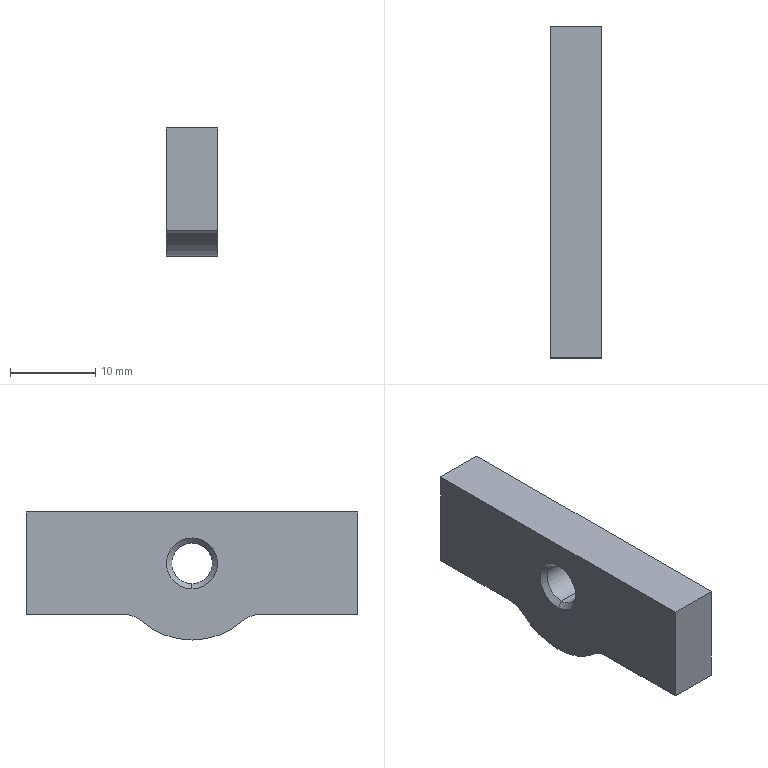Part | STEP file | 2026.6.15-Main Assembly图.sldasm-Part-231 | 1 solid | 17 faces | box 6 x 39 x 15.045 mm | volume 2873 mm3 | plane 7 | cylinder 6 | cone 4 | commonest cylinder face diameters 4.8 x2 6 x2 18 x2
STEP:
#1=CARTESIAN_POINT('',(-1568.238,1430.217,3336.397));
#2=VERTEX_POINT('',#1);
#3=CARTESIAN_POINT('',(-1568.238,1424.264,3334.147));
#4=VERTEX_POINT('',#3);
#5=CARTESIAN_POINT('',(-1568.238,1424.264,3343.147));
#6=DIRECTION('',(-1.,0.,0.));
#7=DIRECTION('',(0.,0.,1.));
#8=AXIS2_PLACEMENT_3D('',#5,#6,#7);
#9=CIRCLE('',#8,9.);
#10=EDGE_CURVE('',#2,#4,#9,.T.);
#11=ORIENTED_EDGE('',*,*,#10,.T.);
#12=CARTESIAN_POINT('',(-1574.238,1424.264,3334.147));
#13=VERTEX_POINT('',#12);
#14=CARTESIAN_POINT('',(-1568.238,1424.264,3334.147));
#15=DIRECTION('',(-1.,0.,0.));
#16=VECTOR('',#15,1000.);
#17=LINE('',#14,#16);
#18=EDGE_CURVE('',#4,#13,#17,.T.);
#19=ORIENTED_EDGE('',*,*,#18,.T.);
#20=CARTESIAN_POINT('',(-1574.238,1430.217,3336.397));
#21=VERTEX_POINT('',#20);
#22=CARTESIAN_POINT('',(-1574.238,1424.264,3343.147));
#23=DIRECTION('',(1.,0.,0.));
#24=DIRECTION('',(0.,0.,1.));
#25=AXIS2_PLACEMENT_3D('',#22,#23,#24);
#26=CIRCLE('',#25,9.);
#27=EDGE_CURVE('',#13,#21,#26,.T.);
#28=ORIENTED_EDGE('',*,*,#27,.T.);
#29=CARTESIAN_POINT('',(-1568.238,1430.217,3336.397));
#30=DIRECTION('',(1.,0.,0.));
#31=VECTOR('',#30,1000.);
#32=LINE('',#29,#31);
#33=EDGE_CURVE('',#21,#2,#32,.T.);
#34=ORIENTED_EDGE('',*,*,#33,.T.);
#35=EDGE_LOOP('',(#11,#19,#28,#34));
#36=FACE_OUTER_BOUND('',#35,.T.);
#37=CARTESIAN_POINT('',(-1568.238,1424.264,3343.147));
#38=DIRECTION('',(-1.,0.,0.));
#39=DIRECTION('',(0.,0.,-1.));
#40=AXIS2_PLACEMENT_3D('',#37,#38,#39);
#41=CYLINDRICAL_SURFACE('',#40,9.);
#42=ADVANCED_FACE('',(#36),#41,.T.);
#43=CARTESIAN_POINT('',(-1568.838,1426.664,3343.147));
#44=VERTEX_POINT('',#43);
#45=CARTESIAN_POINT('',(-1568.238,1427.264,3343.147));
#46=VERTEX_POINT('',#45);
#47=CARTESIAN_POINT('',(-1568.238,1427.264,3343.147));
#48=DIRECTION('',(0.7071,0.7071,0.));
#49=VECTOR('',#48,1000.);
#50=LINE('',#47,#49);
#51=EDGE_CURVE('',#44,#46,#50,.T.);
#52=ORIENTED_EDGE('',*,*,#51,.F.);
#53=CARTESIAN_POINT('',(-1568.838,1424.264,3340.747));
#54=VERTEX_POINT('',#53);
#55=CARTESIAN_POINT('',(-1568.838,1424.264,3343.147));
#56=DIRECTION('',(-1.,0.,0.));
#57=DIRECTION('',(0.,0.,-1.));
#58=AXIS2_PLACEMENT_3D('',#55,#56,#57);
#59=CIRCLE('',#58,2.4);
#60=EDGE_CURVE('',#44,#54,#59,.T.);
#61=ORIENTED_EDGE('',*,*,#60,.T.);
#62=CARTESIAN_POINT('',(-1568.838,1421.864,3343.147));
#63=VERTEX_POINT('',#62);
#64=CARTESIAN_POINT('',(-1568.838,1424.264,3343.147));
#65=DIRECTION('',(-1.,0.,0.));
#66=DIRECTION('',(0.,0.,-1.));
#67=AXIS2_PLACEMENT_3D('',#64,#65,#66);
#68=CIRCLE('',#67,2.4);
#69=EDGE_CURVE('',#54,#63,#68,.T.);
#70=ORIENTED_EDGE('',*,*,#69,.T.);
#71=CARTESIAN_POINT('',(-1568.238,1421.264,3343.147));
#72=VERTEX_POINT('',#71);
#73=CARTESIAN_POINT('',(-1568.238,1421.264,3343.147));
#74=DIRECTION('',(0.7071,-0.7071,0.));
#75=VECTOR('',#74,1000.);
#76=LINE('',#73,#75);
#77=EDGE_CURVE('',#63,#72,#76,.T.);
#78=ORIENTED_EDGE('',*,*,#77,.T.);
#79=CARTESIAN_POINT('',(-1568.238,1424.264,3343.147));
#80=DIRECTION('',(-1.,0.,0.));
#81=DIRECTION('',(0.,-1.,0.));
#82=AXIS2_PLACEMENT_3D('',#79,#80,#81);
#83=CIRCLE('',#82,3.);
#84=EDGE_CURVE('',#46,#72,#83,.T.);
#85=ORIENTED_EDGE('',*,*,#84,.F.);
#86=EDGE_LOOP('',(#52,#61,#70,#78,#85));
#87=FACE_OUTER_BOUND('',#86,.T.);
#88=CARTESIAN_POINT('',(-1568.238,1424.264,3343.147));
#89=DIRECTION('',(1.,0.,0.));
#90=DIRECTION('',(0.,1.,0.));
#91=AXIS2_PLACEMENT_3D('',#88,#89,#90);
#92=CONICAL_SURFACE('',#91,3.,0.7854);
#93=ADVANCED_FACE('',(#87),#92,.F.);
#94=CARTESIAN_POINT('',(-1573.638,1424.264,3345.547));
#95=VERTEX_POINT('',#94);
#96=CARTESIAN_POINT('',(-1568.838,1424.264,3345.547));
#97=VERTEX_POINT('',#96);
#98=CARTESIAN_POINT('',(-1574.238,1424.264,3345.547));
#99=DIRECTION('',(1.,0.,0.));
#100=VECTOR('',#99,1000.);
#101=LINE('',#98,#100);
#102=EDGE_CURVE('',#95,#97,#101,.T.);
#103=ORIENTED_EDGE('',*,*,#102,.F.);
#104=CARTESIAN_POINT('',(-1573.638,1424.264,3340.747));
#105=VERTEX_POINT('',#104);
#106=CARTESIAN_POINT('',(-1573.638,1424.264,3343.147));
#107=DIRECTION('',(-1.,0.,0.));
#108=DIRECTION('',(0.,0.,1.));
#109=AXIS2_PLACEMENT_3D('',#106,#107,#108);
#110=CIRCLE('',#109,2.4);
#111=EDGE_CURVE('',#95,#105,#110,.T.);
#112=ORIENTED_EDGE('',*,*,#111,.T.);
#113=CARTESIAN_POINT('',(-1574.238,1424.264,3340.747));
#114=DIRECTION('',(1.,0.,0.));
#115=VECTOR('',#114,1000.);
#116=LINE('',#113,#115);
#117=EDGE_CURVE('',#105,#54,#116,.T.);
#118=ORIENTED_EDGE('',*,*,#117,.T.);
#119=ORIENTED_EDGE('',*,*,#60,.F.);
#120=CARTESIAN_POINT('',(-1568.838,1424.264,3343.147));
#121=DIRECTION('',(-1.,0.,0.));
#122=DIRECTION('',(0.,0.,-1.));
#123=AXIS2_PLACEMENT_3D('',#120,#121,#122);
#124=CIRCLE('',#123,2.4);
#125=EDGE_CURVE('',#97,#44,#124,.T.);
#126=ORIENTED_EDGE('',*,*,#125,.F.);
#127=EDGE_LOOP('',(#103,#112,#118,#119,#126));
#128=FACE_OUTER_BOUND('',#127,.T.);
#129=CARTESIAN_POINT('',(-1574.238,1424.264,3343.147));
#130=DIRECTION('',(1.,0.,0.));
#131=DIRECTION('',(0.,0.,1.));
#132=AXIS2_PLACEMENT_3D('',#129,#130,#131);
#133=CYLINDRICAL_SURFACE('',#132,2.4);
#134=ADVANCED_FACE('',(#128),#133,.F.);
#135=CARTESIAN_POINT('',(-1568.238,1432.202,3337.147));
#136=VERTEX_POINT('',#135);
#137=CARTESIAN_POINT('',(-1568.238,1443.764,3337.147));
#138=VERTEX_POINT('',#137);
#139=CARTESIAN_POINT('',(-1568.238,1443.764,3337.147));
#140=DIRECTION('',(0.,1.,0.));
#141=VECTOR('',#140,1000.);
#142=LINE('',#139,#141);
#143=EDGE_CURVE('',#136,#138,#142,.T.);
#144=ORIENTED_EDGE('',*,*,#143,.T.);
#145=CARTESIAN_POINT('',(-1568.238,1443.764,3349.192));
#146=VERTEX_POINT('',#145);
#147=CARTESIAN_POINT('',(-1568.238,1443.764,3349.192));
#148=DIRECTION('',(0.,0.,1.));
#149=VECTOR('',#148,1000.);
#150=LINE('',#147,#149);
#151=EDGE_CURVE('',#138,#146,#150,.T.);
#152=ORIENTED_EDGE('',*,*,#151,.T.);
#153=CARTESIAN_POINT('',(-1568.238,1404.764,3349.192));
#154=VERTEX_POINT('',#153);
#155=CARTESIAN_POINT('',(-1568.238,1443.764,3349.192));
#156=DIRECTION('',(0.,-1.,0.));
#157=VECTOR('',#156,1000.);
#158=LINE('',#155,#157);
#159=EDGE_CURVE('',#146,#154,#158,.T.);
#160=ORIENTED_EDGE('',*,*,#159,.T.);
#161=CARTESIAN_POINT('',(-1568.238,1404.764,3337.147));
#162=VERTEX_POINT('',#161);
#163=CARTESIAN_POINT('',(-1568.238,1404.764,3349.192));
#164=DIRECTION('',(0.,0.,-1.));
#165=VECTOR('',#164,1000.);
#166=LINE('',#163,#165);
#167=EDGE_CURVE('',#154,#162,#166,.T.);
#168=ORIENTED_EDGE('',*,*,#167,.T.);
#169=CARTESIAN_POINT('',(-1568.238,1416.327,3337.147));
#170=VERTEX_POINT('',#169);
#171=CARTESIAN_POINT('',(-1568.238,1443.764,3337.147));
#172=DIRECTION('',(0.,1.,0.));
#173=VECTOR('',#172,1000.);
#174=LINE('',#171,#173);
#175=EDGE_CURVE('',#162,#170,#174,.T.);
#176=ORIENTED_EDGE('',*,*,#175,.T.);
#177=CARTESIAN_POINT('',(-1568.238,1418.311,3336.397));
#178=VERTEX_POINT('',#177);
#179=CARTESIAN_POINT('',(-1568.238,1416.327,3334.147));
#180=DIRECTION('',(-1.,0.,0.));
#181=DIRECTION('',(0.,0.,1.));
#182=AXIS2_PLACEMENT_3D('',#179,#180,#181);
#183=CIRCLE('',#182,3.);
#184=EDGE_CURVE('',#170,#178,#183,.T.);
#185=ORIENTED_EDGE('',*,*,#184,.T.);
#186=CARTESIAN_POINT('',(-1568.238,1424.264,3343.147));
#187=DIRECTION('',(-1.,0.,0.));
#188=DIRECTION('',(0.,0.,1.));
#189=AXIS2_PLACEMENT_3D('',#186,#187,#188);
#190=CIRCLE('',#189,9.);
#191=EDGE_CURVE('',#4,#178,#190,.T.);
#192=ORIENTED_EDGE('',*,*,#191,.F.);
#193=ORIENTED_EDGE('',*,*,#10,.F.);
#194=CARTESIAN_POINT('',(-1568.238,1432.202,3334.147));
#195=DIRECTION('',(-1.,0.,0.));
#196=DIRECTION('',(0.,0.,1.));
#197=AXIS2_PLACEMENT_3D('',#194,#195,#196);
#198=CIRCLE('',#197,3.);
#199=EDGE_CURVE('',#2,#136,#198,.T.);
#200=ORIENTED_EDGE('',*,*,#199,.T.);
#201=EDGE_LOOP('',(#144,#152,#160,#168,#176,#185,#192,#193,#200));
#202=FACE_OUTER_BOUND('',#201,.T.);
#203=CARTESIAN_POINT('',(-1568.238,1424.264,3343.147));
#204=DIRECTION('',(-1.,0.,0.));
#205=DIRECTION('',(0.,-1.,0.));
#206=AXIS2_PLACEMENT_3D('',#203,#204,#205);
#207=CIRCLE('',#206,3.);
#208=EDGE_CURVE('',#72,#46,#207,.T.);
#209=ORIENTED_EDGE('',*,*,#208,.T.);
#210=ORIENTED_EDGE('',*,*,#84,.T.);
#211=EDGE_LOOP('',(#209,#210));
#212=FACE_BOUND('',#211,.T.);
#213=CARTESIAN_POINT('',(-1568.238,1424.264,3370.147));
#214=DIRECTION('',(1.,0.,0.));
#215=DIRECTION('',(0.,-1.,0.));
#216=AXIS2_PLACEMENT_3D('',#213,#214,#215);
#217=PLANE('',#216);
#218=ADVANCED_FACE('',(#202,#212),#217,.T.);
#219=CARTESIAN_POINT('',(-1574.238,1424.264,3340.147));
#220=VERTEX_POINT('',#219);
#221=CARTESIAN_POINT('',(-1574.238,1424.264,3340.147));
#222=DIRECTION('',(0.7071,0.,0.7071));
#223=VECTOR('',#222,1000.);
#224=LINE('',#221,#223);
#225=EDGE_CURVE('',#220,#105,#224,.T.);
#226=ORIENTED_EDGE('',*,*,#225,.T.);
#227=ORIENTED_EDGE('',*,*,#111,.F.);
#228=CARTESIAN_POINT('',(-1574.238,1424.264,3346.147));
#229=VERTEX_POINT('',#228);
#230=CARTESIAN_POINT('',(-1574.238,1424.264,3346.147));
#231=DIRECTION('',(0.7071,0.,-0.7071));
#232=VECTOR('',#231,1000.);
#233=LINE('',#230,#232);
#234=EDGE_CURVE('',#229,#95,#233,.T.);
#235=ORIENTED_EDGE('',*,*,#234,.F.);
#236=CARTESIAN_POINT('',(-1574.238,1424.264,3343.147));
#237=DIRECTION('',(-1.,0.,0.));
#238=DIRECTION('',(0.,0.,1.));
#239=AXIS2_PLACEMENT_3D('',#236,#237,#238);
#240=CIRCLE('',#239,3.);
#241=EDGE_CURVE('',#229,#220,#240,.T.);
#242=ORIENTED_EDGE('',*,*,#241,.T.);
#243=EDGE_LOOP('',(#226,#227,#235,#242));
#244=FACE_OUTER_BOUND('',#243,.T.);
#245=CARTESIAN_POINT('',(-1574.238,1424.264,3343.147));
#246=DIRECTION('',(-1.,0.,0.));
#247=DIRECTION('',(0.,0.,-1.));
#248=AXIS2_PLACEMENT_3D('',#245,#246,#247);
#249=CONICAL_SURFACE('',#248,3.,0.7854);
#250=ADVANCED_FACE('',(#244),#249,.F.);
#251=CARTESIAN_POINT('',(-1574.238,1404.764,3349.192));
#252=VERTEX_POINT('',#251);
#253=CARTESIAN_POINT('',(-1574.238,1404.764,3349.192));
#254=DIRECTION('',(-1.,0.,0.));
#255=VECTOR('',#254,1000.);
#256=LINE('',#253,#255);
#257=EDGE_CURVE('',#154,#252,#256,.T.);
#258=ORIENTED_EDGE('',*,*,#257,.T.);
#259=CARTESIAN_POINT('',(-1574.238,1404.764,3337.147));
#260=VERTEX_POINT('',#259);
#261=CARTESIAN_POINT('',(-1574.238,1404.764,3370.147));
#262=DIRECTION('',(0.,0.,-1.));
#263=VECTOR('',#262,1000.);
#264=LINE('',#261,#263);
#265=EDGE_CURVE('',#252,#260,#264,.T.);
#266=ORIENTED_EDGE('',*,*,#265,.T.);
#267=CARTESIAN_POINT('',(-1574.238,1404.764,3337.147));
#268=DIRECTION('',(1.,0.,0.));
#269=VECTOR('',#268,1000.);
#270=LINE('',#267,#269);
#271=EDGE_CURVE('',#260,#162,#270,.T.);
#272=ORIENTED_EDGE('',*,*,#271,.T.);
#273=ORIENTED_EDGE('',*,*,#167,.F.);
#274=EDGE_LOOP('',(#258,#266,#272,#273));
#275=FACE_OUTER_BOUND('',#274,.T.);
#276=CARTESIAN_POINT('',(-1574.238,1404.764,3349.192));
#277=DIRECTION('',(0.,1.,0.));
#278=DIRECTION('',(1.,0.,0.));
#279=AXIS2_PLACEMENT_3D('',#276,#277,#278);
#280=PLANE('',#279);
#281=ADVANCED_FACE('',(#275),#280,.F.);
#282=CARTESIAN_POINT('',(-1574.238,1416.327,3337.147));
#283=VERTEX_POINT('',#282);
#284=CARTESIAN_POINT('',(-1568.238,1416.327,3337.147));
#285=DIRECTION('',(1.,0.,0.));
#286=VECTOR('',#285,1000.);
#287=LINE('',#284,#286);
#288=EDGE_CURVE('',#283,#170,#287,.T.);
#289=ORIENTED_EDGE('',*,*,#288,.T.);
#290=ORIENTED_EDGE('',*,*,#175,.F.);
#291=ORIENTED_EDGE('',*,*,#271,.F.);
#292=CARTESIAN_POINT('',(-1574.238,1424.264,3337.147));
#293=DIRECTION('',(0.,1.,0.));
#294=VECTOR('',#293,1000.);
#295=LINE('',#292,#294);
#296=EDGE_CURVE('',#260,#283,#295,.T.);
#297=ORIENTED_EDGE('',*,*,#296,.T.);
#298=EDGE_LOOP('',(#289,#290,#291,#297));
#299=FACE_OUTER_BOUND('',#298,.T.);
#300=CARTESIAN_POINT('',(-1574.238,1443.764,3337.147));
#301=DIRECTION('',(0.,0.,1.));
#302=DIRECTION('',(-1.,0.,0.));
#303=AXIS2_PLACEMENT_3D('',#300,#301,#302);
#304=PLANE('',#303);
#305=ADVANCED_FACE('',(#299),#304,.F.);
#306=ORIENTED_EDGE('',*,*,#288,.F.);
#307=CARTESIAN_POINT('',(-1574.238,1418.311,3336.397));
#308=VERTEX_POINT('',#307);
#309=CARTESIAN_POINT('',(-1574.238,1416.327,3334.147));
#310=DIRECTION('',(-1.,0.,0.));
#311=DIRECTION('',(0.,0.,1.));
#312=AXIS2_PLACEMENT_3D('',#309,#310,#311);
#313=CIRCLE('',#312,3.);
#314=EDGE_CURVE('',#283,#308,#313,.T.);
#315=ORIENTED_EDGE('',*,*,#314,.T.);
#316=CARTESIAN_POINT('',(-1568.238,1418.311,3336.397));
#317=DIRECTION('',(-1.,0.,0.));
#318=VECTOR('',#317,1000.);
#319=LINE('',#316,#318);
#320=EDGE_CURVE('',#178,#308,#319,.T.);
#321=ORIENTED_EDGE('',*,*,#320,.F.);
#322=ORIENTED_EDGE('',*,*,#184,.F.);
#323=EDGE_LOOP('',(#306,#315,#321,#322));
#324=FACE_OUTER_BOUND('',#323,.T.);
#325=CARTESIAN_POINT('',(-1568.238,1416.327,3334.147));
#326=DIRECTION('',(-1.,0.,0.));
#327=DIRECTION('',(0.,0.,-1.));
#328=AXIS2_PLACEMENT_3D('',#325,#326,#327);
#329=CYLINDRICAL_SURFACE('',#328,3.);
#330=ADVANCED_FACE('',(#324),#329,.F.);
#331=ORIENTED_EDGE('',*,*,#18,.F.);
#332=ORIENTED_EDGE('',*,*,#191,.T.);
#333=ORIENTED_EDGE('',*,*,#320,.T.);
#334=CARTESIAN_POINT('',(-1574.238,1424.264,3343.147));
#335=DIRECTION('',(1.,0.,0.));
#336=DIRECTION('',(0.,0.,1.));
#337=AXIS2_PLACEMENT_3D('',#334,#335,#336);
#338=CIRCLE('',#337,9.);
#339=EDGE_CURVE('',#308,#13,#338,.T.);
#340=ORIENTED_EDGE('',*,*,#339,.T.);
#341=EDGE_LOOP('',(#331,#332,#333,#340));
#342=FACE_OUTER_BOUND('',#341,.T.);
#343=CARTESIAN_POINT('',(-1568.238,1424.264,3343.147));
#344=DIRECTION('',(-1.,0.,0.));
#345=DIRECTION('',(0.,0.,-1.));
#346=AXIS2_PLACEMENT_3D('',#343,#344,#345);
#347=CYLINDRICAL_SURFACE('',#346,9.);
#348=ADVANCED_FACE('',(#342),#347,.T.);
#349=ORIENTED_EDGE('',*,*,#33,.F.);
#350=CARTESIAN_POINT('',(-1574.238,1432.202,3337.147));
#351=VERTEX_POINT('',#350);
#352=CARTESIAN_POINT('',(-1574.238,1432.202,3334.147));
#353=DIRECTION('',(-1.,0.,0.));
#354=DIRECTION('',(0.,0.,1.));
#355=AXIS2_PLACEMENT_3D('',#352,#353,#354);
#356=CIRCLE('',#355,3.);
#357=EDGE_CURVE('',#21,#351,#356,.T.);
#358=ORIENTED_EDGE('',*,*,#357,.T.);
#359=CARTESIAN_POINT('',(-1574.238,1432.202,3337.147));
#360=DIRECTION('',(1.,0.,0.));
#361=VECTOR('',#360,1000.);
#362=LINE('',#359,#361);
#363=EDGE_CURVE('',#351,#136,#362,.T.);
#364=ORIENTED_EDGE('',*,*,#363,.T.);
#365=ORIENTED_EDGE('',*,*,#199,.F.);
#366=EDGE_LOOP('',(#349,#358,#364,#365));
#367=FACE_OUTER_BOUND('',#366,.T.);
#368=CARTESIAN_POINT('',(-1568.238,1432.202,3334.147));
#369=DIRECTION('',(-1.,0.,0.));
#370=DIRECTION('',(0.,0.,-1.));
#371=AXIS2_PLACEMENT_3D('',#368,#369,#370);
#372=CYLINDRICAL_SURFACE('',#371,3.);
#373=ADVANCED_FACE('',(#367),#372,.F.);
#374=ORIENTED_EDGE('',*,*,#363,.F.);
#375=CARTESIAN_POINT('',(-1574.238,1443.764,3337.147));
#376=VERTEX_POINT('',#375);
#377=CARTESIAN_POINT('',(-1574.238,1424.264,3337.147));
#378=DIRECTION('',(0.,1.,0.));
#379=VECTOR('',#378,1000.);
#380=LINE('',#377,#379);
#381=EDGE_CURVE('',#351,#376,#380,.T.);
#382=ORIENTED_EDGE('',*,*,#381,.T.);
#383=CARTESIAN_POINT('',(-1574.238,1443.764,3337.147));
#384=DIRECTION('',(1.,0.,0.));
#385=VECTOR('',#384,1000.);
#386=LINE('',#383,#385);
#387=EDGE_CURVE('',#376,#138,#386,.T.);
#388=ORIENTED_EDGE('',*,*,#387,.T.);
#389=ORIENTED_EDGE('',*,*,#143,.F.);
#390=EDGE_LOOP('',(#374,#382,#388,#389));
#391=FACE_OUTER_BOUND('',#390,.T.);
#392=CARTESIAN_POINT('',(-1574.238,1443.764,3337.147));
#393=DIRECTION('',(0.,0.,1.));
#394=DIRECTION('',(-1.,0.,0.));
#395=AXIS2_PLACEMENT_3D('',#392,#393,#394);
#396=PLANE('',#395);
#397=ADVANCED_FACE('',(#391),#396,.F.);
#398=ORIENTED_EDGE('',*,*,#387,.F.);
#399=CARTESIAN_POINT('',(-1574.238,1443.764,3349.192));
#400=VERTEX_POINT('',#399);
#401=CARTESIAN_POINT('',(-1574.238,1443.764,3370.147));
#402=DIRECTION('',(0.,0.,1.));
#403=VECTOR('',#402,1000.);
#404=LINE('',#401,#403);
#405=EDGE_CURVE('',#376,#400,#404,.T.);
#406=ORIENTED_EDGE('',*,*,#405,.T.);
#407=CARTESIAN_POINT('',(-1574.238,1443.764,3349.192));
#408=DIRECTION('',(1.,0.,0.));
#409=VECTOR('',#408,1000.);
#410=LINE('',#407,#409);
#411=EDGE_CURVE('',#400,#146,#410,.T.);
#412=ORIENTED_EDGE('',*,*,#411,.T.);
#413=ORIENTED_EDGE('',*,*,#151,.F.);
#414=EDGE_LOOP('',(#398,#406,#412,#413));
#415=FACE_OUTER_BOUND('',#414,.T.);
#416=CARTESIAN_POINT('',(-1574.238,1443.764,3349.192));
#417=DIRECTION('',(0.,-1.,0.));
#418=DIRECTION('',(-1.,0.,0.));
#419=AXIS2_PLACEMENT_3D('',#416,#417,#418);
#420=PLANE('',#419);
#421=ADVANCED_FACE('',(#415),#420,.F.);
#422=ORIENTED_EDGE('',*,*,#411,.F.);
#423=CARTESIAN_POINT('',(-1574.238,1424.264,3349.192));
#424=DIRECTION('',(0.,-1.,0.));
#425=VECTOR('',#424,1000.);
#426=LINE('',#423,#425);
#427=EDGE_CURVE('',#400,#252,#426,.T.);
#428=ORIENTED_EDGE('',*,*,#427,.T.);
#429=ORIENTED_EDGE('',*,*,#257,.F.);
#430=ORIENTED_EDGE('',*,*,#159,.F.);
#431=EDGE_LOOP('',(#422,#428,#429,#430));
#432=FACE_OUTER_BOUND('',#431,.T.);
#433=CARTESIAN_POINT('',(-1574.238,1443.764,3349.192));
#434=DIRECTION('',(0.,0.,-1.));
#435=DIRECTION('',(1.,0.,0.));
#436=AXIS2_PLACEMENT_3D('',#433,#434,#435);
#437=PLANE('',#436);
#438=ADVANCED_FACE('',(#432),#437,.F.);
#439=ORIENTED_EDGE('',*,*,#405,.F.);
#440=ORIENTED_EDGE('',*,*,#381,.F.);
#441=ORIENTED_EDGE('',*,*,#357,.F.);
#442=ORIENTED_EDGE('',*,*,#27,.F.);
#443=ORIENTED_EDGE('',*,*,#339,.F.);
#444=ORIENTED_EDGE('',*,*,#314,.F.);
#445=ORIENTED_EDGE('',*,*,#296,.F.);
#446=ORIENTED_EDGE('',*,*,#265,.F.);
#447=ORIENTED_EDGE('',*,*,#427,.F.);
#448=EDGE_LOOP('',(#439,#440,#441,#442,#443,#444,#445,#446,#447));
#449=FACE_OUTER_BOUND('',#448,.T.);
#450=ORIENTED_EDGE('',*,*,#241,.F.);
#451=CARTESIAN_POINT('',(-1574.238,1424.264,3343.147));
#452=DIRECTION('',(-1.,0.,0.));
#453=DIRECTION('',(0.,0.,1.));
#454=AXIS2_PLACEMENT_3D('',#451,#452,#453);
#455=CIRCLE('',#454,3.);
#456=EDGE_CURVE('',#220,#229,#455,.T.);
#457=ORIENTED_EDGE('',*,*,#456,.F.);
#458=EDGE_LOOP('',(#450,#457));
#459=FACE_BOUND('',#458,.T.);
#460=CARTESIAN_POINT('',(-1574.238,1424.264,3370.147));
#461=DIRECTION('',(1.,0.,0.));
#462=DIRECTION('',(0.,-1.,0.));
#463=AXIS2_PLACEMENT_3D('',#460,#461,#462);
#464=PLANE('',#463);
#465=ADVANCED_FACE('',(#449,#459),#464,.F.);
#466=CARTESIAN_POINT('',(-1568.838,1424.264,3343.147));
#467=DIRECTION('',(-1.,0.,0.));
#468=DIRECTION('',(0.,0.,-1.));
#469=AXIS2_PLACEMENT_3D('',#466,#467,#468);
#470=CIRCLE('',#469,2.4);
#471=EDGE_CURVE('',#63,#97,#470,.T.);
#472=ORIENTED_EDGE('',*,*,#471,.T.);
#473=ORIENTED_EDGE('',*,*,#125,.T.);
#474=ORIENTED_EDGE('',*,*,#51,.T.);
#475=ORIENTED_EDGE('',*,*,#208,.F.);
#476=ORIENTED_EDGE('',*,*,#77,.F.);
#477=EDGE_LOOP('',(#472,#473,#474,#475,#476));
#478=FACE_OUTER_BOUND('',#477,.T.);
#479=CARTESIAN_POINT('',(-1568.238,1424.264,3343.147));
#480=DIRECTION('',(1.,0.,0.));
#481=DIRECTION('',(0.,1.,0.));
#482=AXIS2_PLACEMENT_3D('',#479,#480,#481);
#483=CONICAL_SURFACE('',#482,3.,0.7854);
#484=ADVANCED_FACE('',(#478),#483,.F.);
#485=CARTESIAN_POINT('',(-1573.638,1424.264,3343.147));
#486=DIRECTION('',(-1.,0.,0.));
#487=DIRECTION('',(0.,0.,1.));
#488=AXIS2_PLACEMENT_3D('',#485,#486,#487);
#489=CIRCLE('',#488,2.4);
#490=EDGE_CURVE('',#105,#95,#489,.T.);
#491=ORIENTED_EDGE('',*,*,#490,.T.);
#492=ORIENTED_EDGE('',*,*,#102,.T.);
#493=ORIENTED_EDGE('',*,*,#471,.F.);
#494=ORIENTED_EDGE('',*,*,#69,.F.);
#495=ORIENTED_EDGE('',*,*,#117,.F.);
#496=EDGE_LOOP('',(#491,#492,#493,#494,#495));
#497=FACE_OUTER_BOUND('',#496,.T.);
#498=CARTESIAN_POINT('',(-1574.238,1424.264,3343.147));
#499=DIRECTION('',(1.,0.,0.));
#500=DIRECTION('',(0.,0.,1.));
#501=AXIS2_PLACEMENT_3D('',#498,#499,#500);
#502=CYLINDRICAL_SURFACE('',#501,2.4);
#503=ADVANCED_FACE('',(#497),#502,.F.);
#504=ORIENTED_EDGE('',*,*,#490,.F.);
#505=ORIENTED_EDGE('',*,*,#225,.F.);
#506=ORIENTED_EDGE('',*,*,#456,.T.);
#507=ORIENTED_EDGE('',*,*,#234,.T.);
#508=EDGE_LOOP('',(#504,#505,#506,#507));
#509=FACE_OUTER_BOUND('',#508,.T.);
#510=CARTESIAN_POINT('',(-1574.238,1424.264,3343.147));
#511=DIRECTION('',(-1.,0.,0.));
#512=DIRECTION('',(0.,0.,-1.));
#513=AXIS2_PLACEMENT_3D('',#510,#511,#512);
#514=CONICAL_SURFACE('',#513,3.,0.7854);
#515=ADVANCED_FACE('',(#509),#514,.F.);
#516=CLOSED_SHELL('',(#42,#93,#134,#218,#250,#281,#305,#330,#348,#373,#397,#421,#438,#465,#484,#503,#515));
#517=MANIFOLD_SOLID_BREP('',#516);
#518=CARTESIAN_POINT('',(0.,0.,0.));
#519=DIRECTION('',(0.,0.,1.));
#520=DIRECTION('',(1.,0.,0.));
#521=AXIS2_PLACEMENT_3D('',#518,#519,#520);
#522=(LENGTH_UNIT()NAMED_UNIT(*)SI_UNIT(.MILLI.,.METRE.));
#523=UNCERTAINTY_MEASURE_WITH_UNIT(LENGTH_MEASURE(0.00001),#522,'','');
#524=(NAMED_UNIT(*)PLANE_ANGLE_UNIT()SI_UNIT($,.RADIAN.));
#525=(NAMED_UNIT(*)SI_UNIT($,.STERADIAN.)SOLID_ANGLE_UNIT());
#526=(GEOMETRIC_REPRESENTATION_CONTEXT(3)GLOBAL_UNCERTAINTY_ASSIGNED_CONTEXT((#523))GLOBAL_UNIT_ASSIGNED_CONTEXT((#522,#524,#525))REPRESENTATION_CONTEXT('',''));
#527=ADVANCED_BREP_SHAPE_REPRESENTATION('',(#517,#521),#526);